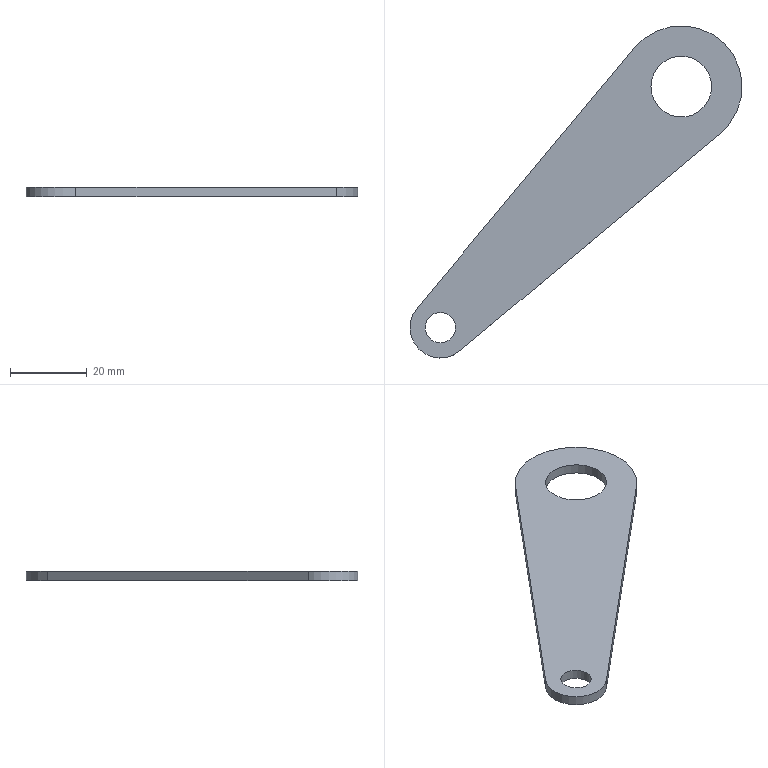Part | NX | features MG0313 aframe 2 | 1 solid | 8 faces | box 86.674 x 86.674 x 2.575 mm | volume 6109 mm3 | plane 4 | cylinder 4 | commonest cylinder face diameters 15.875 x2 7.938 x1 31.75 x1
STEP:
#1=CARTESIAN_POINT('',(-58.893,-62.862,105.762));
#2=VERTEX_POINT('',#1);
#3=CARTESIAN_POINT('',(-62.862,-62.862,105.762));
#4=DIRECTION('',(0.,0.,1.));
#5=DIRECTION('',(1.,0.,0.));
#6=AXIS2_PLACEMENT_3D('',#3,#4,#5);
#7=CIRCLE('',#6,3.969);
#8=EDGE_CURVE('',#2,#2,#7,.T.);
#9=ORIENTED_EDGE('',*,*,#8,.F.);
#10=EDGE_LOOP('',(#9));
#11=FACE_BOUND('',#10,.T.);
#12=CARTESIAN_POINT('',(-68.953,-57.773,105.762));
#13=VERTEX_POINT('',#12);
#14=CARTESIAN_POINT('',(-57.773,-68.953,105.762));
#15=VERTEX_POINT('',#14);
#16=CARTESIAN_POINT('',(-62.862,-62.862,105.762));
#17=DIRECTION('',(0.,0.,1.));
#18=DIRECTION('',(1.,0.,0.));
#19=AXIS2_PLACEMENT_3D('',#16,#17,#18);
#20=CIRCLE('',#19,7.938);
#21=EDGE_CURVE('',#13,#15,#20,.T.);
#22=ORIENTED_EDGE('',*,*,#21,.T.);
#23=CARTESIAN_POINT('',(10.178,-12.183,105.762));
#24=VERTEX_POINT('',#23);
#25=CARTESIAN_POINT('',(10.178,-12.183,105.762));
#26=DIRECTION('',(0.7674,0.6411,0.));
#27=VECTOR('',#26,1000.);
#28=LINE('',#25,#27);
#29=EDGE_CURVE('',#15,#24,#28,.T.);
#30=ORIENTED_EDGE('',*,*,#29,.T.);
#31=CARTESIAN_POINT('',(-12.183,10.178,105.762));
#32=VERTEX_POINT('',#31);
#33=CARTESIAN_POINT('',(0.,0.,105.762));
#34=DIRECTION('',(0.,0.,1.));
#35=DIRECTION('',(1.,0.,0.));
#36=AXIS2_PLACEMENT_3D('',#33,#34,#35);
#37=CIRCLE('',#36,15.875);
#38=EDGE_CURVE('',#24,#32,#37,.T.);
#39=ORIENTED_EDGE('',*,*,#38,.T.);
#40=CARTESIAN_POINT('',(-68.953,-57.773,105.762));
#41=DIRECTION('',(-0.6411,-0.7674,0.));
#42=VECTOR('',#41,1000.);
#43=LINE('',#40,#42);
#44=EDGE_CURVE('',#32,#13,#43,.T.);
#45=ORIENTED_EDGE('',*,*,#44,.T.);
#46=EDGE_LOOP('',(#22,#30,#39,#45));
#47=FACE_BOUND('',#46,.T.);
#48=CARTESIAN_POINT('',(7.938,0.,105.762));
#49=VERTEX_POINT('',#48);
#50=CARTESIAN_POINT('',(0.,0.,105.762));
#51=DIRECTION('',(0.,0.,1.));
#52=DIRECTION('',(1.,0.,0.));
#53=AXIS2_PLACEMENT_3D('',#50,#51,#52);
#54=CIRCLE('',#53,7.938);
#55=EDGE_CURVE('',#49,#49,#54,.T.);
#56=ORIENTED_EDGE('',*,*,#55,.F.);
#57=EDGE_LOOP('',(#56));
#58=FACE_BOUND('',#57,.T.);
#59=CARTESIAN_POINT('',(-62.862,-62.862,105.762));
#60=DIRECTION('',(0.,0.,1.));
#61=DIRECTION('',(1.,0.,0.));
#62=AXIS2_PLACEMENT_3D('',#59,#60,#61);
#63=PLANE('',#62);
#64=ADVANCED_FACE('',(#11,#47,#58),#63,.T.);
#65=CARTESIAN_POINT('',(-58.893,-62.862,103.188));
#66=VERTEX_POINT('',#65);
#67=CARTESIAN_POINT('',(-62.862,-62.862,103.188));
#68=DIRECTION('',(0.,0.,1.));
#69=DIRECTION('',(1.,0.,0.));
#70=AXIS2_PLACEMENT_3D('',#67,#68,#69);
#71=CIRCLE('',#70,3.969);
#72=EDGE_CURVE('',#66,#66,#71,.T.);
#73=ORIENTED_EDGE('',*,*,#72,.T.);
#74=EDGE_LOOP('',(#73));
#75=FACE_BOUND('',#74,.T.);
#76=CARTESIAN_POINT('',(-68.953,-57.773,103.188));
#77=VERTEX_POINT('',#76);
#78=CARTESIAN_POINT('',(-57.773,-68.953,103.188));
#79=VERTEX_POINT('',#78);
#80=CARTESIAN_POINT('',(-62.862,-62.862,103.188));
#81=DIRECTION('',(0.,0.,1.));
#82=DIRECTION('',(1.,0.,0.));
#83=AXIS2_PLACEMENT_3D('',#80,#81,#82);
#84=CIRCLE('',#83,7.938);
#85=EDGE_CURVE('',#77,#79,#84,.T.);
#86=ORIENTED_EDGE('',*,*,#85,.F.);
#87=CARTESIAN_POINT('',(-12.183,10.178,103.188));
#88=VERTEX_POINT('',#87);
#89=CARTESIAN_POINT('',(-68.953,-57.773,103.188));
#90=DIRECTION('',(-0.6411,-0.7674,0.));
#91=VECTOR('',#90,1000.);
#92=LINE('',#89,#91);
#93=EDGE_CURVE('',#88,#77,#92,.T.);
#94=ORIENTED_EDGE('',*,*,#93,.F.);
#95=CARTESIAN_POINT('',(10.178,-12.183,103.188));
#96=VERTEX_POINT('',#95);
#97=CARTESIAN_POINT('',(0.,0.,103.188));
#98=DIRECTION('',(0.,0.,1.));
#99=DIRECTION('',(1.,0.,0.));
#100=AXIS2_PLACEMENT_3D('',#97,#98,#99);
#101=CIRCLE('',#100,15.875);
#102=EDGE_CURVE('',#96,#88,#101,.T.);
#103=ORIENTED_EDGE('',*,*,#102,.F.);
#104=CARTESIAN_POINT('',(10.178,-12.183,103.188));
#105=DIRECTION('',(0.7674,0.6411,0.));
#106=VECTOR('',#105,1000.);
#107=LINE('',#104,#106);
#108=EDGE_CURVE('',#79,#96,#107,.T.);
#109=ORIENTED_EDGE('',*,*,#108,.F.);
#110=EDGE_LOOP('',(#86,#94,#103,#109));
#111=FACE_BOUND('',#110,.T.);
#112=CARTESIAN_POINT('',(7.938,0.,103.188));
#113=VERTEX_POINT('',#112);
#114=CARTESIAN_POINT('',(0.,0.,103.188));
#115=DIRECTION('',(0.,0.,1.));
#116=DIRECTION('',(1.,0.,0.));
#117=AXIS2_PLACEMENT_3D('',#114,#115,#116);
#118=CIRCLE('',#117,7.938);
#119=EDGE_CURVE('',#113,#113,#118,.T.);
#120=ORIENTED_EDGE('',*,*,#119,.T.);
#121=EDGE_LOOP('',(#120));
#122=FACE_BOUND('',#121,.T.);
#123=CARTESIAN_POINT('',(-62.862,-62.862,103.188));
#124=DIRECTION('',(0.,0.,1.));
#125=DIRECTION('',(1.,0.,0.));
#126=AXIS2_PLACEMENT_3D('',#123,#124,#125);
#127=PLANE('',#126);
#128=ADVANCED_FACE('',(#75,#111,#122),#127,.F.);
#129=ORIENTED_EDGE('',*,*,#85,.T.);
#130=CARTESIAN_POINT('',(-57.773,-68.953,104.762));
#131=DIRECTION('',(0.,0.,-1.));
#132=VECTOR('',#131,1000.);
#133=LINE('',#130,#132);
#134=EDGE_CURVE('',#15,#79,#133,.T.);
#135=ORIENTED_EDGE('',*,*,#134,.F.);
#136=ORIENTED_EDGE('',*,*,#21,.F.);
#137=CARTESIAN_POINT('',(-68.953,-57.773,104.762));
#138=DIRECTION('',(0.,0.,-1.));
#139=VECTOR('',#138,1000.);
#140=LINE('',#137,#139);
#141=EDGE_CURVE('',#13,#77,#140,.T.);
#142=ORIENTED_EDGE('',*,*,#141,.T.);
#143=EDGE_LOOP('',(#129,#135,#136,#142));
#144=FACE_BOUND('',#143,.T.);
#145=CARTESIAN_POINT('',(-62.862,-62.862,104.762));
#146=DIRECTION('',(0.,0.,-1.));
#147=DIRECTION('',(-1.,0.,0.));
#148=AXIS2_PLACEMENT_3D('',#145,#146,#147);
#149=CYLINDRICAL_SURFACE('',#148,7.938);
#150=ADVANCED_FACE('',(#144),#149,.T.);
#151=ORIENTED_EDGE('',*,*,#108,.T.);
#152=CARTESIAN_POINT('',(10.178,-12.183,104.762));
#153=DIRECTION('',(0.,0.,-1.));
#154=VECTOR('',#153,1000.);
#155=LINE('',#152,#154);
#156=EDGE_CURVE('',#24,#96,#155,.T.);
#157=ORIENTED_EDGE('',*,*,#156,.F.);
#158=ORIENTED_EDGE('',*,*,#29,.F.);
#159=ORIENTED_EDGE('',*,*,#134,.T.);
#160=EDGE_LOOP('',(#151,#157,#158,#159));
#161=FACE_BOUND('',#160,.T.);
#162=CARTESIAN_POINT('',(10.178,-12.183,104.762));
#163=DIRECTION('',(-0.6411,0.7674,0.));
#164=DIRECTION('',(-0.7674,-0.6411,0.));
#165=AXIS2_PLACEMENT_3D('',#162,#163,#164);
#166=PLANE('',#165);
#167=ADVANCED_FACE('',(#161),#166,.F.);
#168=ORIENTED_EDGE('',*,*,#102,.T.);
#169=CARTESIAN_POINT('',(-12.183,10.178,104.762));
#170=DIRECTION('',(0.,0.,-1.));
#171=VECTOR('',#170,1000.);
#172=LINE('',#169,#171);
#173=EDGE_CURVE('',#32,#88,#172,.T.);
#174=ORIENTED_EDGE('',*,*,#173,.F.);
#175=ORIENTED_EDGE('',*,*,#38,.F.);
#176=ORIENTED_EDGE('',*,*,#156,.T.);
#177=EDGE_LOOP('',(#168,#174,#175,#176));
#178=FACE_BOUND('',#177,.T.);
#179=CARTESIAN_POINT('',(0.,0.,104.762));
#180=DIRECTION('',(0.,0.,-1.));
#181=DIRECTION('',(-1.,0.,0.));
#182=AXIS2_PLACEMENT_3D('',#179,#180,#181);
#183=CYLINDRICAL_SURFACE('',#182,15.875);
#184=ADVANCED_FACE('',(#178),#183,.T.);
#185=ORIENTED_EDGE('',*,*,#93,.T.);
#186=ORIENTED_EDGE('',*,*,#141,.F.);
#187=ORIENTED_EDGE('',*,*,#44,.F.);
#188=ORIENTED_EDGE('',*,*,#173,.T.);
#189=EDGE_LOOP('',(#185,#186,#187,#188));
#190=FACE_BOUND('',#189,.T.);
#191=CARTESIAN_POINT('',(-68.953,-57.773,104.762));
#192=DIRECTION('',(0.7674,-0.6411,0.));
#193=DIRECTION('',(0.6411,0.7674,0.));
#194=AXIS2_PLACEMENT_3D('',#191,#192,#193);
#195=PLANE('',#194);
#196=ADVANCED_FACE('',(#190),#195,.F.);
#197=ORIENTED_EDGE('',*,*,#8,.T.);
#198=EDGE_LOOP('',(#197));
#199=FACE_BOUND('',#198,.T.);
#200=ORIENTED_EDGE('',*,*,#72,.F.);
#201=EDGE_LOOP('',(#200));
#202=FACE_BOUND('',#201,.T.);
#203=CARTESIAN_POINT('',(-62.862,-62.862,104.762));
#204=DIRECTION('',(0.,0.,-1.));
#205=DIRECTION('',(-1.,0.,0.));
#206=AXIS2_PLACEMENT_3D('',#203,#204,#205);
#207=CYLINDRICAL_SURFACE('',#206,3.969);
#208=ADVANCED_FACE('',(#199,#202),#207,.F.);
#209=ORIENTED_EDGE('',*,*,#55,.T.);
#210=EDGE_LOOP('',(#209));
#211=FACE_BOUND('',#210,.T.);
#212=ORIENTED_EDGE('',*,*,#119,.F.);
#213=EDGE_LOOP('',(#212));
#214=FACE_BOUND('',#213,.T.);
#215=CARTESIAN_POINT('',(0.,0.,104.762));
#216=DIRECTION('',(0.,0.,-1.));
#217=DIRECTION('',(-1.,0.,0.));
#218=AXIS2_PLACEMENT_3D('',#215,#216,#217);
#219=CYLINDRICAL_SURFACE('',#218,7.938);
#220=ADVANCED_FACE('',(#211,#214),#219,.F.);
#221=CLOSED_SHELL('',(#64,#128,#150,#167,#184,#196,#208,#220));
#222=MANIFOLD_SOLID_BREP('',#221);
#223=(LENGTH_UNIT()NAMED_UNIT(*)SI_UNIT(.MILLI.,.METRE.));
#224=UNCERTAINTY_MEASURE_WITH_UNIT(LENGTH_MEASURE(0.00001),#223,'','');
#225=(NAMED_UNIT(*)PLANE_ANGLE_UNIT()SI_UNIT($,.RADIAN.));
#226=(NAMED_UNIT(*)SI_UNIT($,.STERADIAN.)SOLID_ANGLE_UNIT());
#227=(GEOMETRIC_REPRESENTATION_CONTEXT(3)GLOBAL_UNCERTAINTY_ASSIGNED_CONTEXT((#224))GLOBAL_UNIT_ASSIGNED_CONTEXT((#223,#225,#226))REPRESENTATION_CONTEXT('',''));
#228=ADVANCED_BREP_SHAPE_REPRESENTATION('',(#222),#227);